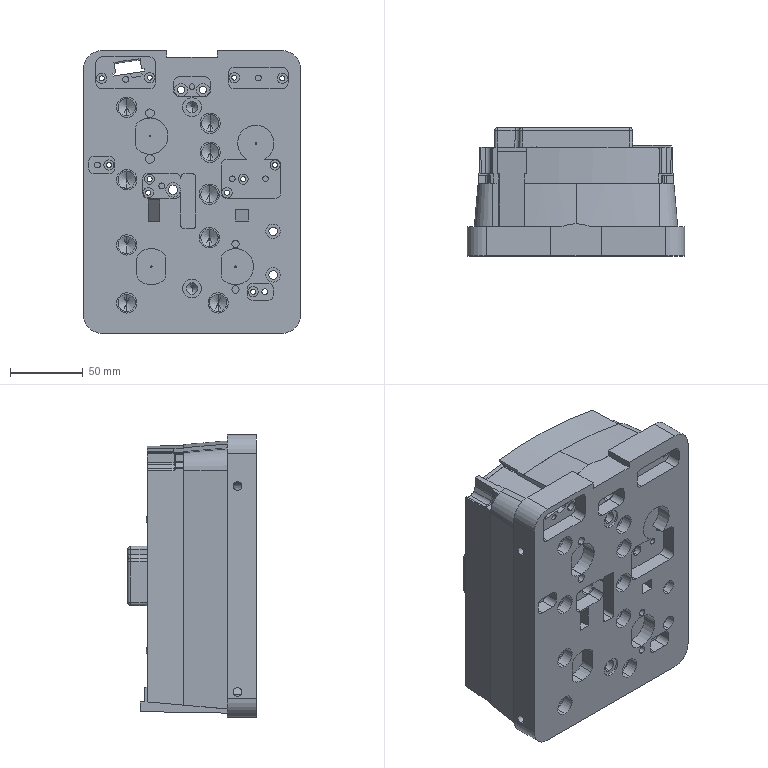Part | STEP file | 1 solid | 693 faces | box 150 x 88.701 x 195 mm | volume 1700421 mm3 | cylinder 308 | plane 286 | cone 71 | spline 11 | torus 10 | sphere 7 | commonest cylinder face diameters 8 x36 6 x35 3.5 x22 4 x22 7 x22 12 x21